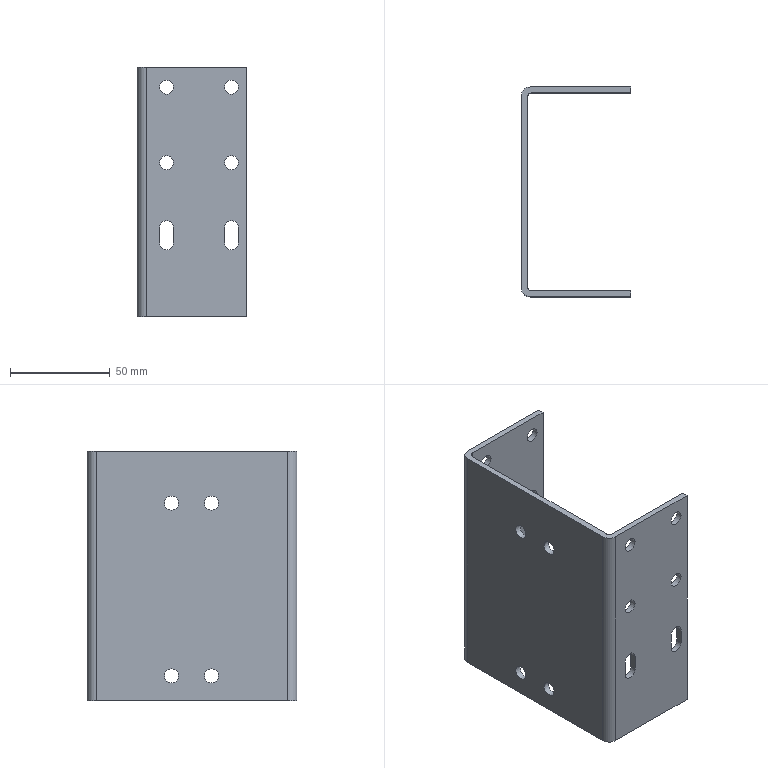Part | STEP file | JIS G 3350A - 1053     40x40x40-100 | 1 solid | 42 faces | box 55 x 105 x 125 mm | volume 75030 mm3 | cylinder 24 | plane 18 | commonest cylinder face diameters 7 x20 4.6 x2 9.2 x2